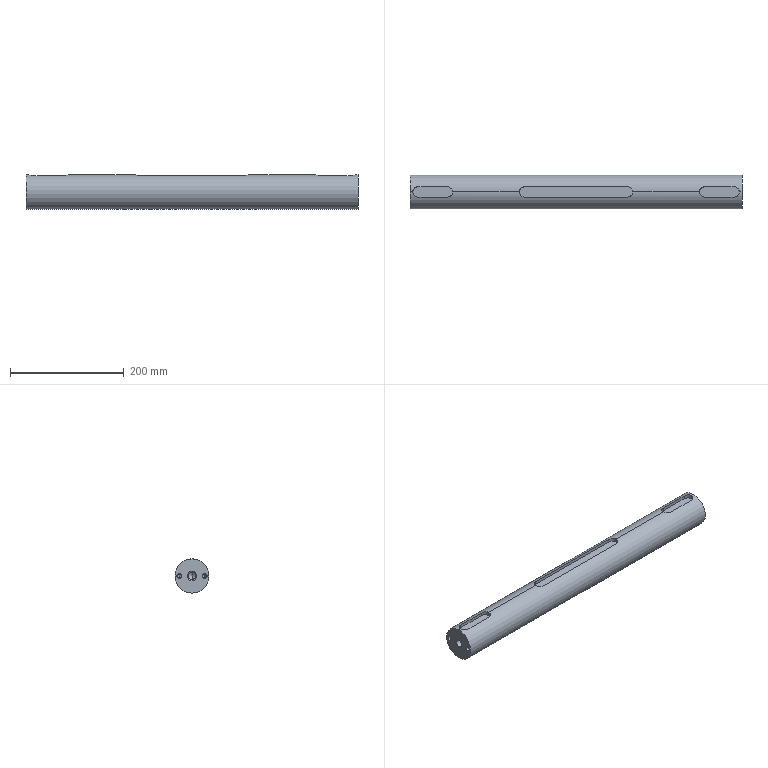Part | SolidWorks | features MBimport 1 | 1 solid | 52 faces | box 584 x 60 x 60 mm | volume 1598343 mm3 | cylinder 23 | cone 16 | plane 13 | commonest cylinder face diameters 18 x9 6.8 x4 8 x4 14 x4 60 x2